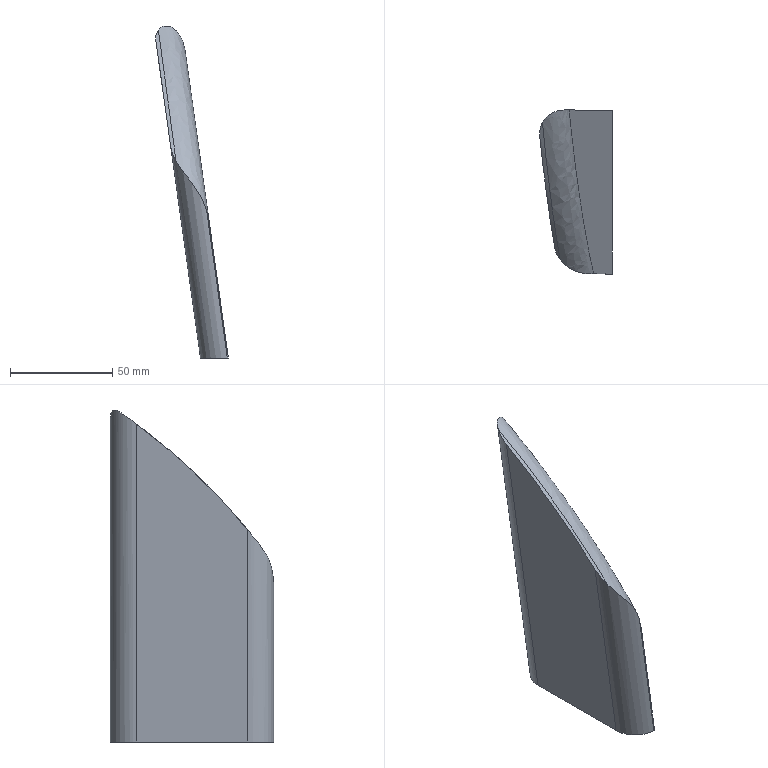Part | STEP file | solid 78 | 1 solid | 9 faces | box 35.54 x 80 x 162.326 mm | volume 129819 mm3 | plane 5 | cylinder 2 | other 1 | spline 1 | commonest cylinder face diameters 26 x2